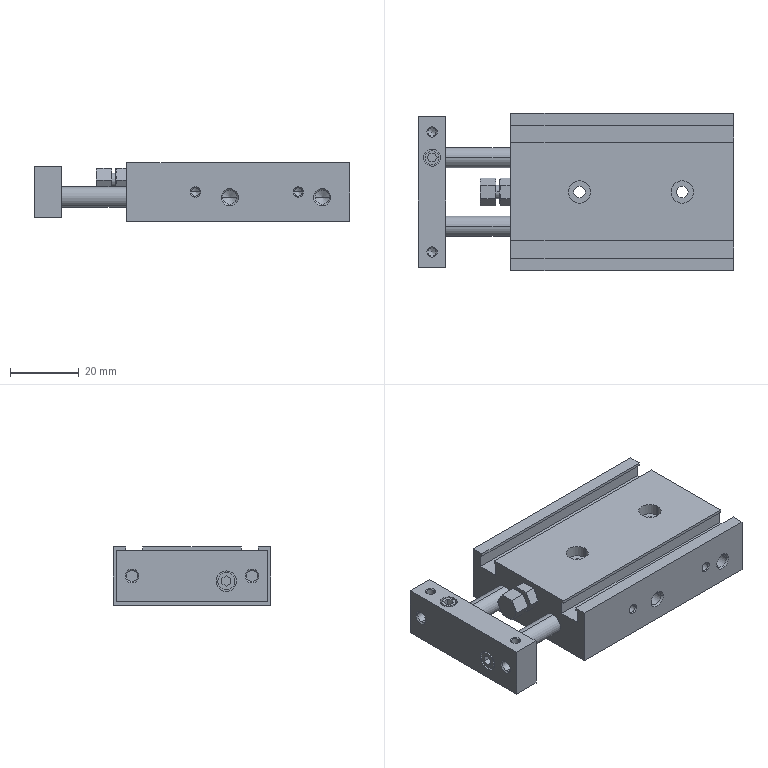Part | SolidWorks | features BaseBody 2, MoveFace 1 | 2 solids | 218 faces | box 92 x 46 x 17 mm | volume 51092 mm3 | cone 85 | plane 71 | cylinder 62 | commonest cylinder face diameters 2.459 x16 6 x10 4.134 x8 10 x8 3.242 x4 3.4 x4